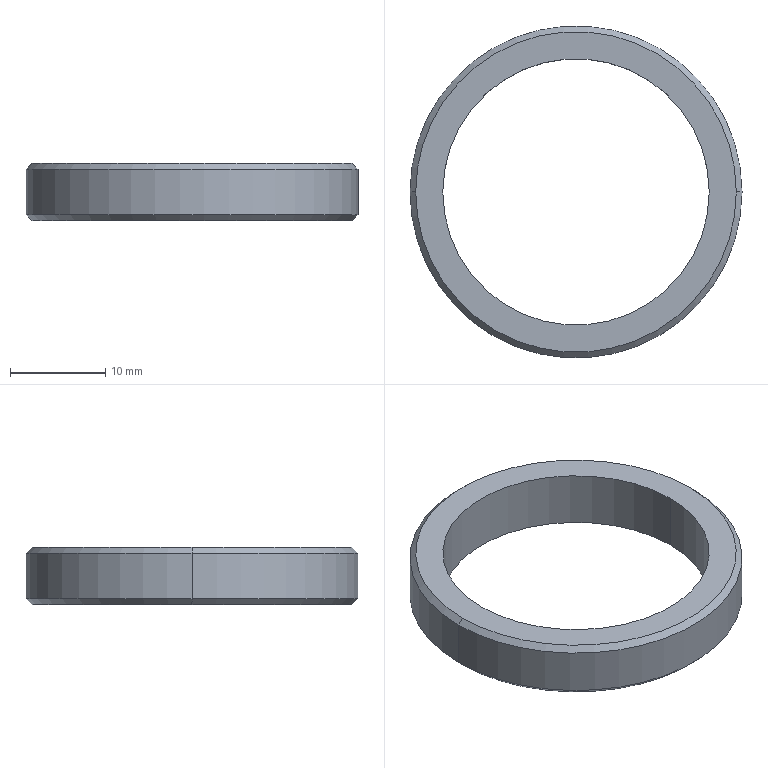Part | STEP file | ESPACIADOR POLEA | 1 solid | 10 faces | box 34.9 x 34.9 x 6 mm | volume 2006 mm3 | cone 4 | cylinder 4 | plane 2 | commonest cylinder face diameters 28 x2 34.9 x2
STEP:
#1=CARTESIAN_POINT('',(16.85,0.,3.));
#2=VERTEX_POINT('',#1);
#3=CARTESIAN_POINT('',(-16.85,0.,3.));
#4=VERTEX_POINT('',#3);
#5=CARTESIAN_POINT('',(0.,0.,3.));
#6=DIRECTION('',(0.,0.,1.));
#7=DIRECTION('',(1.,0.,0.));
#8=AXIS2_PLACEMENT_3D('',#5,#6,#7);
#9=CIRCLE('',#8,16.85);
#10=EDGE_CURVE('',#2,#4,#9,.T.);
#11=ORIENTED_EDGE('',*,*,#10,.F.);
#12=CARTESIAN_POINT('',(17.45,0.,2.4));
#13=VERTEX_POINT('',#12);
#14=CARTESIAN_POINT('',(16.85,0.,3.));
#15=DIRECTION('',(0.7071,0.,-0.7071));
#16=VECTOR('',#15,1000.);
#17=LINE('',#14,#16);
#18=EDGE_CURVE('',#2,#13,#17,.T.);
#19=ORIENTED_EDGE('',*,*,#18,.T.);
#20=CARTESIAN_POINT('',(-17.45,0.,2.4));
#21=VERTEX_POINT('',#20);
#22=CARTESIAN_POINT('',(0.,0.,2.4));
#23=DIRECTION('',(0.,0.,-1.));
#24=DIRECTION('',(1.,0.,0.));
#25=AXIS2_PLACEMENT_3D('',#22,#23,#24);
#26=CIRCLE('',#25,17.45);
#27=EDGE_CURVE('',#21,#13,#26,.T.);
#28=ORIENTED_EDGE('',*,*,#27,.F.);
#29=CARTESIAN_POINT('',(-16.85,0.,3.));
#30=DIRECTION('',(-0.7071,0.,-0.7071));
#31=VECTOR('',#30,1000.);
#32=LINE('',#29,#31);
#33=EDGE_CURVE('',#4,#21,#32,.T.);
#34=ORIENTED_EDGE('',*,*,#33,.F.);
#35=EDGE_LOOP('',(#11,#19,#28,#34));
#36=FACE_OUTER_BOUND('',#35,.T.);
#37=CARTESIAN_POINT('',(0.,0.,3.));
#38=DIRECTION('',(0.,0.,-1.));
#39=DIRECTION('',(-1.,0.,0.));
#40=AXIS2_PLACEMENT_3D('',#37,#38,#39);
#41=CONICAL_SURFACE('',#40,16.85,0.7854);
#42=ADVANCED_FACE('',(#36),#41,.T.);
#43=CARTESIAN_POINT('',(-16.85,0.,-3.));
#44=VERTEX_POINT('',#43);
#45=CARTESIAN_POINT('',(16.85,0.,-3.));
#46=VERTEX_POINT('',#45);
#47=CARTESIAN_POINT('',(0.,0.,-3.));
#48=DIRECTION('',(0.,0.,-1.));
#49=DIRECTION('',(1.,0.,0.));
#50=AXIS2_PLACEMENT_3D('',#47,#48,#49);
#51=CIRCLE('',#50,16.85);
#52=EDGE_CURVE('',#44,#46,#51,.T.);
#53=ORIENTED_EDGE('',*,*,#52,.F.);
#54=CARTESIAN_POINT('',(-17.45,0.,-2.4));
#55=VERTEX_POINT('',#54);
#56=CARTESIAN_POINT('',(-17.45,0.,-2.4));
#57=DIRECTION('',(-0.7071,0.,0.7071));
#58=VECTOR('',#57,1000.);
#59=LINE('',#56,#58);
#60=EDGE_CURVE('',#44,#55,#59,.T.);
#61=ORIENTED_EDGE('',*,*,#60,.T.);
#62=CARTESIAN_POINT('',(17.45,0.,-2.4));
#63=VERTEX_POINT('',#62);
#64=CARTESIAN_POINT('',(0.,0.,-2.4));
#65=DIRECTION('',(0.,0.,1.));
#66=DIRECTION('',(1.,0.,0.));
#67=AXIS2_PLACEMENT_3D('',#64,#65,#66);
#68=CIRCLE('',#67,17.45);
#69=EDGE_CURVE('',#63,#55,#68,.T.);
#70=ORIENTED_EDGE('',*,*,#69,.F.);
#71=CARTESIAN_POINT('',(17.45,0.,-2.4));
#72=DIRECTION('',(0.7071,0.,0.7071));
#73=VECTOR('',#72,1000.);
#74=LINE('',#71,#73);
#75=EDGE_CURVE('',#46,#63,#74,.T.);
#76=ORIENTED_EDGE('',*,*,#75,.F.);
#77=EDGE_LOOP('',(#53,#61,#70,#76));
#78=FACE_OUTER_BOUND('',#77,.T.);
#79=CARTESIAN_POINT('',(0.,0.,-2.4));
#80=DIRECTION('',(0.,0.,1.));
#81=DIRECTION('',(1.,0.,0.));
#82=AXIS2_PLACEMENT_3D('',#79,#80,#81);
#83=CONICAL_SURFACE('',#82,17.45,0.7854);
#84=ADVANCED_FACE('',(#78),#83,.T.);
#85=CARTESIAN_POINT('',(-14.,0.,3.));
#86=VERTEX_POINT('',#85);
#87=CARTESIAN_POINT('',(14.,0.,3.));
#88=VERTEX_POINT('',#87);
#89=CARTESIAN_POINT('',(0.,0.,3.));
#90=DIRECTION('',(0.,0.,1.));
#91=DIRECTION('',(1.,0.,0.));
#92=AXIS2_PLACEMENT_3D('',#89,#90,#91);
#93=CIRCLE('',#92,14.);
#94=EDGE_CURVE('',#86,#88,#93,.T.);
#95=ORIENTED_EDGE('',*,*,#94,.T.);
#96=CARTESIAN_POINT('',(14.,0.,-3.));
#97=VERTEX_POINT('',#96);
#98=CARTESIAN_POINT('',(14.,0.,3.));
#99=DIRECTION('',(0.,0.,-1.));
#100=VECTOR('',#99,1000.);
#101=LINE('',#98,#100);
#102=EDGE_CURVE('',#88,#97,#101,.T.);
#103=ORIENTED_EDGE('',*,*,#102,.T.);
#104=CARTESIAN_POINT('',(-14.,0.,-3.));
#105=VERTEX_POINT('',#104);
#106=CARTESIAN_POINT('',(0.,0.,-3.));
#107=DIRECTION('',(0.,0.,1.));
#108=DIRECTION('',(1.,0.,0.));
#109=AXIS2_PLACEMENT_3D('',#106,#107,#108);
#110=CIRCLE('',#109,14.);
#111=EDGE_CURVE('',#105,#97,#110,.T.);
#112=ORIENTED_EDGE('',*,*,#111,.F.);
#113=CARTESIAN_POINT('',(-14.,0.,3.));
#114=DIRECTION('',(0.,0.,-1.));
#115=VECTOR('',#114,1000.);
#116=LINE('',#113,#115);
#117=EDGE_CURVE('',#86,#105,#116,.T.);
#118=ORIENTED_EDGE('',*,*,#117,.F.);
#119=EDGE_LOOP('',(#95,#103,#112,#118));
#120=FACE_OUTER_BOUND('',#119,.T.);
#121=CARTESIAN_POINT('',(0.,0.,3.));
#122=DIRECTION('',(0.,0.,-1.));
#123=DIRECTION('',(-1.,0.,0.));
#124=AXIS2_PLACEMENT_3D('',#121,#122,#123);
#125=CYLINDRICAL_SURFACE('',#124,14.);
#126=ADVANCED_FACE('',(#120),#125,.F.);
#127=ORIENTED_EDGE('',*,*,#27,.T.);
#128=CARTESIAN_POINT('',(17.45,0.,3.));
#129=DIRECTION('',(0.,0.,-1.));
#130=VECTOR('',#129,1000.);
#131=LINE('',#128,#130);
#132=EDGE_CURVE('',#13,#63,#131,.T.);
#133=ORIENTED_EDGE('',*,*,#132,.T.);
#134=ORIENTED_EDGE('',*,*,#69,.T.);
#135=CARTESIAN_POINT('',(-17.45,0.,3.));
#136=DIRECTION('',(0.,0.,-1.));
#137=VECTOR('',#136,1000.);
#138=LINE('',#135,#137);
#139=EDGE_CURVE('',#21,#55,#138,.T.);
#140=ORIENTED_EDGE('',*,*,#139,.F.);
#141=EDGE_LOOP('',(#127,#133,#134,#140));
#142=FACE_OUTER_BOUND('',#141,.T.);
#143=CARTESIAN_POINT('',(0.,0.,3.));
#144=DIRECTION('',(0.,0.,-1.));
#145=DIRECTION('',(-1.,0.,0.));
#146=AXIS2_PLACEMENT_3D('',#143,#144,#145);
#147=CYLINDRICAL_SURFACE('',#146,17.45);
#148=ADVANCED_FACE('',(#142),#147,.T.);
#149=CARTESIAN_POINT('',(0.,0.,3.));
#150=DIRECTION('',(0.,0.,1.));
#151=DIRECTION('',(1.,0.,0.));
#152=AXIS2_PLACEMENT_3D('',#149,#150,#151);
#153=CIRCLE('',#152,16.85);
#154=EDGE_CURVE('',#4,#2,#153,.T.);
#155=ORIENTED_EDGE('',*,*,#154,.T.);
#156=ORIENTED_EDGE('',*,*,#10,.T.);
#157=EDGE_LOOP('',(#155,#156));
#158=FACE_OUTER_BOUND('',#157,.T.);
#159=ORIENTED_EDGE('',*,*,#94,.F.);
#160=CARTESIAN_POINT('',(0.,0.,3.));
#161=DIRECTION('',(0.,0.,1.));
#162=DIRECTION('',(1.,0.,0.));
#163=AXIS2_PLACEMENT_3D('',#160,#161,#162);
#164=CIRCLE('',#163,14.);
#165=EDGE_CURVE('',#88,#86,#164,.T.);
#166=ORIENTED_EDGE('',*,*,#165,.F.);
#167=EDGE_LOOP('',(#159,#166));
#168=FACE_BOUND('',#167,.T.);
#169=CARTESIAN_POINT('',(0.,0.,3.));
#170=DIRECTION('',(0.,0.,1.));
#171=DIRECTION('',(1.,0.,0.));
#172=AXIS2_PLACEMENT_3D('',#169,#170,#171);
#173=PLANE('',#172);
#174=ADVANCED_FACE('',(#158,#168),#173,.T.);
#175=CARTESIAN_POINT('',(0.,0.,-3.));
#176=DIRECTION('',(0.,0.,-1.));
#177=DIRECTION('',(1.,0.,0.));
#178=AXIS2_PLACEMENT_3D('',#175,#176,#177);
#179=CIRCLE('',#178,16.85);
#180=EDGE_CURVE('',#46,#44,#179,.T.);
#181=ORIENTED_EDGE('',*,*,#180,.T.);
#182=ORIENTED_EDGE('',*,*,#52,.T.);
#183=EDGE_LOOP('',(#181,#182));
#184=FACE_OUTER_BOUND('',#183,.T.);
#185=ORIENTED_EDGE('',*,*,#111,.T.);
#186=CARTESIAN_POINT('',(0.,0.,-3.));
#187=DIRECTION('',(0.,0.,1.));
#188=DIRECTION('',(1.,0.,0.));
#189=AXIS2_PLACEMENT_3D('',#186,#187,#188);
#190=CIRCLE('',#189,14.);
#191=EDGE_CURVE('',#97,#105,#190,.T.);
#192=ORIENTED_EDGE('',*,*,#191,.T.);
#193=EDGE_LOOP('',(#185,#192));
#194=FACE_BOUND('',#193,.T.);
#195=CARTESIAN_POINT('',(0.,0.,-3.));
#196=DIRECTION('',(0.,0.,1.));
#197=DIRECTION('',(1.,0.,0.));
#198=AXIS2_PLACEMENT_3D('',#195,#196,#197);
#199=PLANE('',#198);
#200=ADVANCED_FACE('',(#184,#194),#199,.F.);
#201=ORIENTED_EDGE('',*,*,#132,.F.);
#202=CARTESIAN_POINT('',(0.,0.,2.4));
#203=DIRECTION('',(0.,0.,-1.));
#204=DIRECTION('',(1.,0.,0.));
#205=AXIS2_PLACEMENT_3D('',#202,#203,#204);
#206=CIRCLE('',#205,17.45);
#207=EDGE_CURVE('',#13,#21,#206,.T.);
#208=ORIENTED_EDGE('',*,*,#207,.T.);
#209=ORIENTED_EDGE('',*,*,#139,.T.);
#210=CARTESIAN_POINT('',(0.,0.,-2.4));
#211=DIRECTION('',(0.,0.,1.));
#212=DIRECTION('',(1.,0.,0.));
#213=AXIS2_PLACEMENT_3D('',#210,#211,#212);
#214=CIRCLE('',#213,17.45);
#215=EDGE_CURVE('',#55,#63,#214,.T.);
#216=ORIENTED_EDGE('',*,*,#215,.T.);
#217=EDGE_LOOP('',(#201,#208,#209,#216));
#218=FACE_OUTER_BOUND('',#217,.T.);
#219=CARTESIAN_POINT('',(0.,0.,3.));
#220=DIRECTION('',(0.,0.,-1.));
#221=DIRECTION('',(-1.,0.,0.));
#222=AXIS2_PLACEMENT_3D('',#219,#220,#221);
#223=CYLINDRICAL_SURFACE('',#222,17.45);
#224=ADVANCED_FACE('',(#218),#223,.T.);
#225=ORIENTED_EDGE('',*,*,#102,.F.);
#226=ORIENTED_EDGE('',*,*,#165,.T.);
#227=ORIENTED_EDGE('',*,*,#117,.T.);
#228=ORIENTED_EDGE('',*,*,#191,.F.);
#229=EDGE_LOOP('',(#225,#226,#227,#228));
#230=FACE_OUTER_BOUND('',#229,.T.);
#231=CARTESIAN_POINT('',(0.,0.,3.));
#232=DIRECTION('',(0.,0.,-1.));
#233=DIRECTION('',(-1.,0.,0.));
#234=AXIS2_PLACEMENT_3D('',#231,#232,#233);
#235=CYLINDRICAL_SURFACE('',#234,14.);
#236=ADVANCED_FACE('',(#230),#235,.F.);
#237=ORIENTED_EDGE('',*,*,#60,.F.);
#238=ORIENTED_EDGE('',*,*,#180,.F.);
#239=ORIENTED_EDGE('',*,*,#75,.T.);
#240=ORIENTED_EDGE('',*,*,#215,.F.);
#241=EDGE_LOOP('',(#237,#238,#239,#240));
#242=FACE_OUTER_BOUND('',#241,.T.);
#243=CARTESIAN_POINT('',(0.,0.,-2.4));
#244=DIRECTION('',(0.,0.,1.));
#245=DIRECTION('',(1.,0.,0.));
#246=AXIS2_PLACEMENT_3D('',#243,#244,#245);
#247=CONICAL_SURFACE('',#246,17.45,0.7854);
#248=ADVANCED_FACE('',(#242),#247,.T.);
#249=ORIENTED_EDGE('',*,*,#18,.F.);
#250=ORIENTED_EDGE('',*,*,#154,.F.);
#251=ORIENTED_EDGE('',*,*,#33,.T.);
#252=ORIENTED_EDGE('',*,*,#207,.F.);
#253=EDGE_LOOP('',(#249,#250,#251,#252));
#254=FACE_OUTER_BOUND('',#253,.T.);
#255=CARTESIAN_POINT('',(0.,0.,3.));
#256=DIRECTION('',(0.,0.,-1.));
#257=DIRECTION('',(-1.,0.,0.));
#258=AXIS2_PLACEMENT_3D('',#255,#256,#257);
#259=CONICAL_SURFACE('',#258,16.85,0.7854);
#260=ADVANCED_FACE('',(#254),#259,.T.);
#261=CLOSED_SHELL('',(#42,#84,#126,#148,#174,#200,#224,#236,#248,#260));
#262=MANIFOLD_SOLID_BREP('',#261);
#263=CARTESIAN_POINT('',(0.,0.,0.));
#264=DIRECTION('',(0.,0.,1.));
#265=DIRECTION('',(1.,0.,0.));
#266=AXIS2_PLACEMENT_3D('',#263,#264,#265);
#267=(LENGTH_UNIT()NAMED_UNIT(*)SI_UNIT(.MILLI.,.METRE.));
#268=UNCERTAINTY_MEASURE_WITH_UNIT(LENGTH_MEASURE(0.00001),#267,'','');
#269=(NAMED_UNIT(*)PLANE_ANGLE_UNIT()SI_UNIT($,.RADIAN.));
#270=(NAMED_UNIT(*)SI_UNIT($,.STERADIAN.)SOLID_ANGLE_UNIT());
#271=(GEOMETRIC_REPRESENTATION_CONTEXT(3)GLOBAL_UNCERTAINTY_ASSIGNED_CONTEXT((#268))GLOBAL_UNIT_ASSIGNED_CONTEXT((#267,#269,#270))REPRESENTATION_CONTEXT('',''));
#272=ADVANCED_BREP_SHAPE_REPRESENTATION('',(#262,#266),#271);